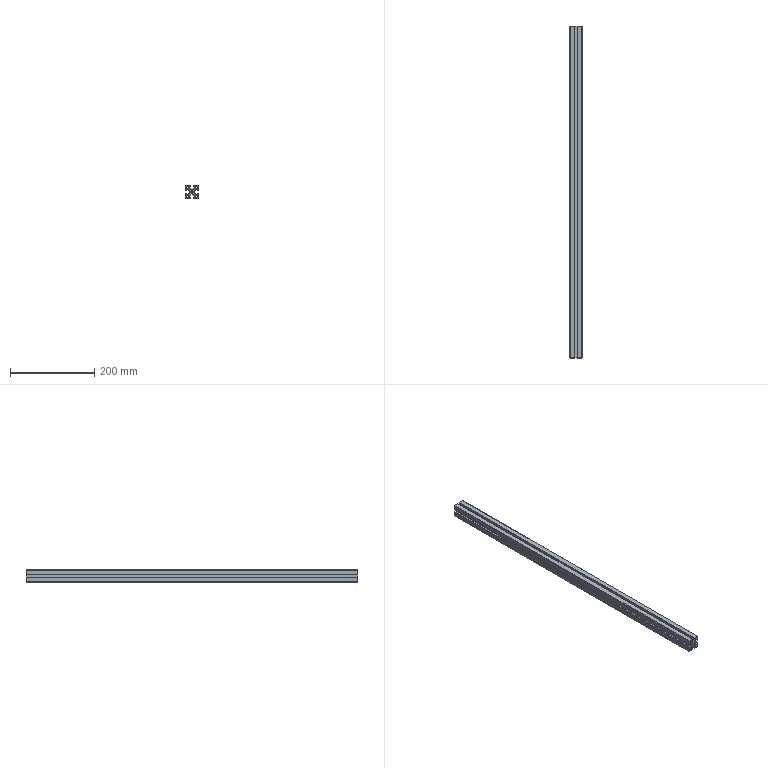Part | STEP file | 08-03 Guard bracket 3 | 1 solid | 68 faces | box 30 x 790 x 30 mm | volume 333958 mm3 | plane 54 | cylinder 14 | commonest cylinder face diameters 6 x10 2 x4